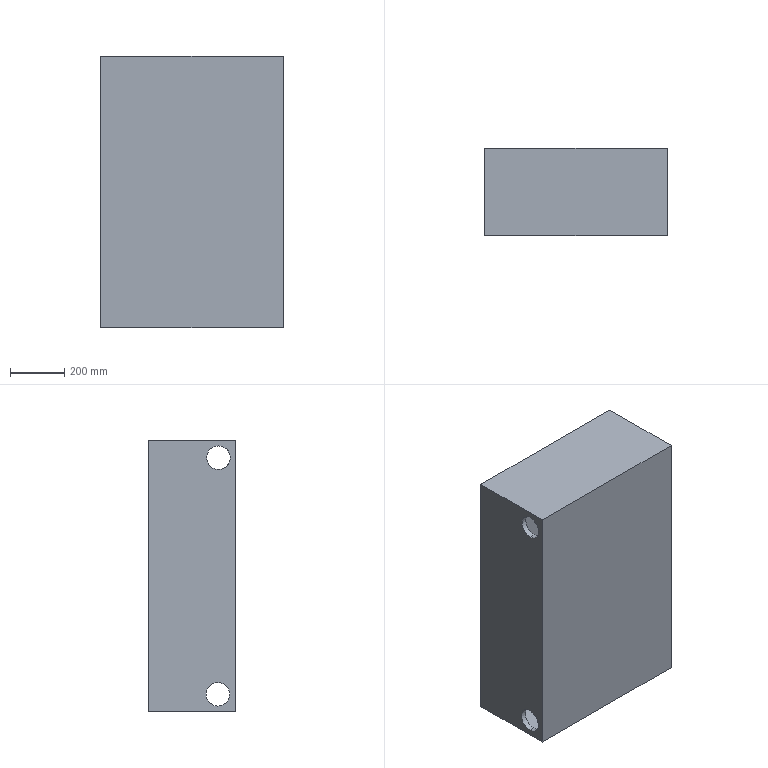Part | SolidWorks | features BaseBody 1 | 1 solid | 34 faces | box 670 x 320 x 1000 mm | volume 50005072 mm3 | cylinder 17 | plane 17 | commonest cylinder face diameters 60 x8 86.602 x7 110 x2
STEP:
#1=CARTESIAN_POINT('',(3055.278,1085.583,108.301));
#2=VERTEX_POINT('',#1);
#3=CARTESIAN_POINT('',(3055.278,1085.583,21.699));
#4=VERTEX_POINT('',#3);
#5=CARTESIAN_POINT('',(3055.278,1085.583,65.));
#6=DIRECTION('',(1.,0.,0.));
#7=DIRECTION('',(0.,0.,-1.));
#8=AXIS2_PLACEMENT_3D('',#5,#6,#7);
#9=CIRCLE('',#8,43.301);
#10=EDGE_CURVE('',#2,#4,#9,.T.);
#11=ORIENTED_EDGE('',*,*,#10,.T.);
#12=CARTESIAN_POINT('',(3035.278,1085.583,21.699));
#13=VERTEX_POINT('',#12);
#14=CARTESIAN_POINT('',(3705.278,1085.583,21.699));
#15=DIRECTION('',(-1.,0.,0.));
#16=VECTOR('',#15,1000.);
#17=LINE('',#14,#16);
#18=EDGE_CURVE('',#4,#13,#17,.T.);
#19=ORIENTED_EDGE('',*,*,#18,.T.);
#20=CARTESIAN_POINT('',(3035.278,1085.583,108.301));
#21=VERTEX_POINT('',#20);
#22=CARTESIAN_POINT('',(3035.278,1085.583,65.));
#23=DIRECTION('',(-1.,0.,0.));
#24=DIRECTION('',(0.,0.,1.));
#25=AXIS2_PLACEMENT_3D('',#22,#23,#24);
#26=CIRCLE('',#25,43.301);
#27=EDGE_CURVE('',#13,#21,#26,.T.);
#28=ORIENTED_EDGE('',*,*,#27,.T.);
#29=CARTESIAN_POINT('',(3705.278,1085.583,108.301));
#30=DIRECTION('',(-1.,0.,0.));
#31=VECTOR('',#30,1000.);
#32=LINE('',#29,#31);
#33=EDGE_CURVE('',#2,#21,#32,.T.);
#34=ORIENTED_EDGE('',*,*,#33,.F.);
#35=EDGE_LOOP('',(#11,#19,#28,#34));
#36=FACE_OUTER_BOUND('',#35,.T.);
#37=CARTESIAN_POINT('',(3705.278,1085.583,65.));
#38=DIRECTION('',(-1.,0.,0.));
#39=DIRECTION('',(0.,0.,1.));
#40=AXIS2_PLACEMENT_3D('',#37,#38,#39);
#41=CYLINDRICAL_SURFACE('',#40,43.301);
#42=ADVANCED_FACE('',(#36),#41,.F.);
#43=CARTESIAN_POINT('',(3705.278,1085.583,21.699));
#44=VERTEX_POINT('',#43);
#45=CARTESIAN_POINT('',(3705.278,1085.583,108.301));
#46=VERTEX_POINT('',#45);
#47=CARTESIAN_POINT('',(3705.278,1085.583,65.));
#48=DIRECTION('',(-1.,0.,0.));
#49=DIRECTION('',(0.,0.,1.));
#50=AXIS2_PLACEMENT_3D('',#47,#48,#49);
#51=CIRCLE('',#50,43.301);
#52=EDGE_CURVE('',#44,#46,#51,.T.);
#53=ORIENTED_EDGE('',*,*,#52,.F.);
#54=CARTESIAN_POINT('',(3685.278,1085.583,21.699));
#55=VERTEX_POINT('',#54);
#56=CARTESIAN_POINT('',(3705.278,1085.583,21.699));
#57=DIRECTION('',(-1.,0.,0.));
#58=VECTOR('',#57,1000.);
#59=LINE('',#56,#58);
#60=EDGE_CURVE('',#44,#55,#59,.T.);
#61=ORIENTED_EDGE('',*,*,#60,.T.);
#62=CARTESIAN_POINT('',(3685.278,1085.583,108.301));
#63=VERTEX_POINT('',#62);
#64=CARTESIAN_POINT('',(3685.278,1085.583,65.));
#65=DIRECTION('',(-1.,0.,0.));
#66=DIRECTION('',(0.,0.,1.));
#67=AXIS2_PLACEMENT_3D('',#64,#65,#66);
#68=CIRCLE('',#67,43.301);
#69=EDGE_CURVE('',#55,#63,#68,.T.);
#70=ORIENTED_EDGE('',*,*,#69,.T.);
#71=CARTESIAN_POINT('',(3705.278,1085.583,108.301));
#72=DIRECTION('',(-1.,0.,0.));
#73=VECTOR('',#72,1000.);
#74=LINE('',#71,#73);
#75=EDGE_CURVE('',#46,#63,#74,.T.);
#76=ORIENTED_EDGE('',*,*,#75,.F.);
#77=EDGE_LOOP('',(#53,#61,#70,#76));
#78=FACE_OUTER_BOUND('',#77,.T.);
#79=CARTESIAN_POINT('',(3705.278,1085.583,65.));
#80=DIRECTION('',(-1.,0.,0.));
#81=DIRECTION('',(0.,0.,1.));
#82=AXIS2_PLACEMENT_3D('',#79,#80,#81);
#83=CYLINDRICAL_SURFACE('',#82,43.301);
#84=ADVANCED_FACE('',(#78),#83,.F.);
#85=CARTESIAN_POINT('',(3705.278,1083.32,891.699));
#86=VERTEX_POINT('',#85);
#87=CARTESIAN_POINT('',(3705.278,1083.32,978.301));
#88=VERTEX_POINT('',#87);
#89=CARTESIAN_POINT('',(3705.278,1083.32,935.));
#90=DIRECTION('',(-1.,0.,0.));
#91=DIRECTION('',(0.,0.,1.));
#92=AXIS2_PLACEMENT_3D('',#89,#90,#91);
#93=CIRCLE('',#92,43.301);
#94=EDGE_CURVE('',#86,#88,#93,.T.);
#95=ORIENTED_EDGE('',*,*,#94,.F.);
#96=CARTESIAN_POINT('',(3685.278,1083.32,891.699));
#97=VERTEX_POINT('',#96);
#98=CARTESIAN_POINT('',(3705.278,1083.32,891.699));
#99=DIRECTION('',(-1.,0.,0.));
#100=VECTOR('',#99,1000.);
#101=LINE('',#98,#100);
#102=EDGE_CURVE('',#86,#97,#101,.T.);
#103=ORIENTED_EDGE('',*,*,#102,.T.);
#104=CARTESIAN_POINT('',(3685.278,1040.583,928.037));
#105=VERTEX_POINT('',#104);
#106=CARTESIAN_POINT('',(3685.278,1083.32,935.));
#107=DIRECTION('',(-1.,0.,0.));
#108=DIRECTION('',(0.,0.,1.));
#109=AXIS2_PLACEMENT_3D('',#106,#107,#108);
#110=CIRCLE('',#109,43.301);
#111=EDGE_CURVE('',#97,#105,#110,.T.);
#112=ORIENTED_EDGE('',*,*,#111,.T.);
#113=CARTESIAN_POINT('',(3055.278,1040.583,928.037));
#114=VERTEX_POINT('',#113);
#115=CARTESIAN_POINT('',(3705.278,1040.583,928.037));
#116=DIRECTION('',(-1.,0.,0.));
#117=VECTOR('',#116,1000.);
#118=LINE('',#115,#117);
#119=EDGE_CURVE('',#105,#114,#118,.T.);
#120=ORIENTED_EDGE('',*,*,#119,.T.);
#121=CARTESIAN_POINT('',(3055.278,1083.32,891.699));
#122=VERTEX_POINT('',#121);
#123=CARTESIAN_POINT('',(3055.278,1083.32,935.));
#124=DIRECTION('',(1.,0.,0.));
#125=DIRECTION('',(0.,0.,-1.));
#126=AXIS2_PLACEMENT_3D('',#123,#124,#125);
#127=CIRCLE('',#126,43.301);
#128=EDGE_CURVE('',#114,#122,#127,.T.);
#129=ORIENTED_EDGE('',*,*,#128,.T.);
#130=CARTESIAN_POINT('',(3035.278,1083.32,891.699));
#131=VERTEX_POINT('',#130);
#132=CARTESIAN_POINT('',(3705.278,1083.32,891.699));
#133=DIRECTION('',(-1.,0.,0.));
#134=VECTOR('',#133,1000.);
#135=LINE('',#132,#134);
#136=EDGE_CURVE('',#122,#131,#135,.T.);
#137=ORIENTED_EDGE('',*,*,#136,.T.);
#138=CARTESIAN_POINT('',(3035.278,1083.32,978.301));
#139=VERTEX_POINT('',#138);
#140=CARTESIAN_POINT('',(3035.278,1083.32,935.));
#141=DIRECTION('',(-1.,0.,0.));
#142=DIRECTION('',(0.,0.,1.));
#143=AXIS2_PLACEMENT_3D('',#140,#141,#142);
#144=CIRCLE('',#143,43.301);
#145=EDGE_CURVE('',#131,#139,#144,.T.);
#146=ORIENTED_EDGE('',*,*,#145,.T.);
#147=CARTESIAN_POINT('',(3055.278,1083.32,978.301));
#148=VERTEX_POINT('',#147);
#149=CARTESIAN_POINT('',(3705.278,1083.32,978.301));
#150=DIRECTION('',(-1.,0.,0.));
#151=VECTOR('',#150,1000.);
#152=LINE('',#149,#151);
#153=EDGE_CURVE('',#148,#139,#152,.T.);
#154=ORIENTED_EDGE('',*,*,#153,.F.);
#155=CARTESIAN_POINT('',(3055.278,1040.583,941.963));
#156=VERTEX_POINT('',#155);
#157=CARTESIAN_POINT('',(3055.278,1083.32,935.));
#158=DIRECTION('',(1.,0.,0.));
#159=DIRECTION('',(0.,0.,-1.));
#160=AXIS2_PLACEMENT_3D('',#157,#158,#159);
#161=CIRCLE('',#160,43.301);
#162=EDGE_CURVE('',#148,#156,#161,.T.);
#163=ORIENTED_EDGE('',*,*,#162,.T.);
#164=CARTESIAN_POINT('',(3685.278,1040.583,941.963));
#165=VERTEX_POINT('',#164);
#166=CARTESIAN_POINT('',(3705.278,1040.583,941.963));
#167=DIRECTION('',(1.,0.,0.));
#168=VECTOR('',#167,1000.);
#169=LINE('',#166,#168);
#170=EDGE_CURVE('',#156,#165,#169,.T.);
#171=ORIENTED_EDGE('',*,*,#170,.T.);
#172=CARTESIAN_POINT('',(3685.278,1083.32,978.301));
#173=VERTEX_POINT('',#172);
#174=CARTESIAN_POINT('',(3685.278,1083.32,935.));
#175=DIRECTION('',(-1.,0.,0.));
#176=DIRECTION('',(0.,0.,1.));
#177=AXIS2_PLACEMENT_3D('',#174,#175,#176);
#178=CIRCLE('',#177,43.301);
#179=EDGE_CURVE('',#165,#173,#178,.T.);
#180=ORIENTED_EDGE('',*,*,#179,.T.);
#181=CARTESIAN_POINT('',(3705.278,1083.32,978.301));
#182=DIRECTION('',(-1.,0.,0.));
#183=VECTOR('',#182,1000.);
#184=LINE('',#181,#183);
#185=EDGE_CURVE('',#88,#173,#184,.T.);
#186=ORIENTED_EDGE('',*,*,#185,.F.);
#187=EDGE_LOOP('',(#95,#103,#112,#120,#129,#137,#146,#154,#163,#171,#180,#186));
#188=FACE_OUTER_BOUND('',#187,.T.);
#189=CARTESIAN_POINT('',(3705.278,1083.32,935.));
#190=DIRECTION('',(-1.,0.,0.));
#191=DIRECTION('',(0.,0.,1.));
#192=AXIS2_PLACEMENT_3D('',#189,#190,#191);
#193=CYLINDRICAL_SURFACE('',#192,43.301);
#194=ADVANCED_FACE('',(#188),#193,.F.);
#195=ORIENTED_EDGE('',*,*,#102,.F.);
#196=CARTESIAN_POINT('',(3705.278,1083.32,935.));
#197=DIRECTION('',(-1.,0.,0.));
#198=DIRECTION('',(0.,0.,1.));
#199=AXIS2_PLACEMENT_3D('',#196,#197,#198);
#200=CIRCLE('',#199,43.301);
#201=EDGE_CURVE('',#88,#86,#200,.T.);
#202=ORIENTED_EDGE('',*,*,#201,.F.);
#203=ORIENTED_EDGE('',*,*,#185,.T.);
#204=CARTESIAN_POINT('',(3685.278,1083.32,935.));
#205=DIRECTION('',(-1.,0.,0.));
#206=DIRECTION('',(0.,0.,1.));
#207=AXIS2_PLACEMENT_3D('',#204,#205,#206);
#208=CIRCLE('',#207,43.301);
#209=EDGE_CURVE('',#173,#97,#208,.T.);
#210=ORIENTED_EDGE('',*,*,#209,.T.);
#211=EDGE_LOOP('',(#195,#202,#203,#210));
#212=FACE_OUTER_BOUND('',#211,.T.);
#213=CARTESIAN_POINT('',(3705.278,1083.32,935.));
#214=DIRECTION('',(-1.,0.,0.));
#215=DIRECTION('',(0.,0.,1.));
#216=AXIS2_PLACEMENT_3D('',#213,#214,#215);
#217=CYLINDRICAL_SURFACE('',#216,43.301);
#218=ADVANCED_FACE('',(#212),#217,.F.);
#219=CARTESIAN_POINT('',(3115.278,1310.583,950.));
#220=VERTEX_POINT('',#219);
#221=CARTESIAN_POINT('',(3055.278,1310.583,950.));
#222=VERTEX_POINT('',#221);
#223=CARTESIAN_POINT('',(3085.278,1310.583,950.));
#224=DIRECTION('',(0.,1.,0.));
#225=DIRECTION('',(-1.,0.,0.));
#226=AXIS2_PLACEMENT_3D('',#223,#224,#225);
#227=CIRCLE('',#226,30.);
#228=EDGE_CURVE('',#220,#222,#227,.T.);
#229=ORIENTED_EDGE('',*,*,#228,.F.);
#230=CARTESIAN_POINT('',(3115.278,1340.583,950.));
#231=VERTEX_POINT('',#230);
#232=CARTESIAN_POINT('',(3115.278,1310.583,950.));
#233=DIRECTION('',(0.,1.,0.));
#234=VECTOR('',#233,1000.);
#235=LINE('',#232,#234);
#236=EDGE_CURVE('',#220,#231,#235,.T.);
#237=ORIENTED_EDGE('',*,*,#236,.T.);
#238=CARTESIAN_POINT('',(3055.278,1340.583,950.));
#239=VERTEX_POINT('',#238);
#240=CARTESIAN_POINT('',(3085.278,1340.583,950.));
#241=DIRECTION('',(0.,1.,0.));
#242=DIRECTION('',(-1.,0.,0.));
#243=AXIS2_PLACEMENT_3D('',#240,#241,#242);
#244=CIRCLE('',#243,30.);
#245=EDGE_CURVE('',#231,#239,#244,.T.);
#246=ORIENTED_EDGE('',*,*,#245,.T.);
#247=CARTESIAN_POINT('',(3055.278,1310.583,950.));
#248=DIRECTION('',(0.,1.,0.));
#249=VECTOR('',#248,1000.);
#250=LINE('',#247,#249);
#251=EDGE_CURVE('',#222,#239,#250,.T.);
#252=ORIENTED_EDGE('',*,*,#251,.F.);
#253=EDGE_LOOP('',(#229,#237,#246,#252));
#254=FACE_OUTER_BOUND('',#253,.T.);
#255=CARTESIAN_POINT('',(3085.278,1310.583,950.));
#256=DIRECTION('',(0.,1.,0.));
#257=DIRECTION('',(-1.,0.,0.));
#258=AXIS2_PLACEMENT_3D('',#255,#256,#257);
#259=CYLINDRICAL_SURFACE('',#258,30.);
#260=ADVANCED_FACE('',(#254),#259,.F.);
#261=CARTESIAN_POINT('',(3685.278,1310.583,50.));
#262=VERTEX_POINT('',#261);
#263=CARTESIAN_POINT('',(3655.278,1310.583,20.));
#264=VERTEX_POINT('',#263);
#265=CARTESIAN_POINT('',(3655.278,1310.583,50.));
#266=DIRECTION('',(0.,1.,0.));
#267=DIRECTION('',(1.,0.,0.));
#268=AXIS2_PLACEMENT_3D('',#265,#266,#267);
#269=CIRCLE('',#268,30.);
#270=EDGE_CURVE('',#262,#264,#269,.T.);
#271=ORIENTED_EDGE('',*,*,#270,.F.);
#272=CARTESIAN_POINT('',(3685.278,1340.583,50.));
#273=VERTEX_POINT('',#272);
#274=CARTESIAN_POINT('',(3685.278,1310.583,50.));
#275=DIRECTION('',(0.,1.,0.));
#276=VECTOR('',#275,1000.);
#277=LINE('',#274,#276);
#278=EDGE_CURVE('',#262,#273,#277,.T.);
#279=ORIENTED_EDGE('',*,*,#278,.T.);
#280=CARTESIAN_POINT('',(3625.278,1340.583,50.));
#281=VERTEX_POINT('',#280);
#282=CARTESIAN_POINT('',(3655.278,1340.583,50.));
#283=DIRECTION('',(0.,1.,0.));
#284=DIRECTION('',(1.,0.,0.));
#285=AXIS2_PLACEMENT_3D('',#282,#283,#284);
#286=CIRCLE('',#285,30.);
#287=EDGE_CURVE('',#273,#281,#286,.T.);
#288=ORIENTED_EDGE('',*,*,#287,.T.);
#289=CARTESIAN_POINT('',(3625.278,1310.583,50.));
#290=VERTEX_POINT('',#289);
#291=CARTESIAN_POINT('',(3625.278,1310.583,50.));
#292=DIRECTION('',(0.,1.,0.));
#293=VECTOR('',#292,1000.);
#294=LINE('',#291,#293);
#295=EDGE_CURVE('',#290,#281,#294,.T.);
#296=ORIENTED_EDGE('',*,*,#295,.F.);
#297=CARTESIAN_POINT('',(3655.278,1310.583,50.));
#298=DIRECTION('',(0.,1.,0.));
#299=DIRECTION('',(1.,0.,0.));
#300=AXIS2_PLACEMENT_3D('',#297,#298,#299);
#301=CIRCLE('',#300,30.);
#302=EDGE_CURVE('',#264,#290,#301,.T.);
#303=ORIENTED_EDGE('',*,*,#302,.F.);
#304=EDGE_LOOP('',(#271,#279,#288,#296,#303));
#305=FACE_OUTER_BOUND('',#304,.T.);
#306=CARTESIAN_POINT('',(3655.278,1310.583,50.));
#307=DIRECTION('',(0.,1.,0.));
#308=DIRECTION('',(-1.,0.,0.));
#309=AXIS2_PLACEMENT_3D('',#306,#307,#308);
#310=CYLINDRICAL_SURFACE('',#309,30.);
#311=ADVANCED_FACE('',(#305),#310,.F.);
#312=CARTESIAN_POINT('',(3685.278,1310.583,950.));
#313=VERTEX_POINT('',#312);
#314=CARTESIAN_POINT('',(3625.278,1310.583,950.));
#315=VERTEX_POINT('',#314);
#316=CARTESIAN_POINT('',(3655.278,1310.583,950.));
#317=DIRECTION('',(0.,1.,0.));
#318=DIRECTION('',(-1.,0.,0.));
#319=AXIS2_PLACEMENT_3D('',#316,#317,#318);
#320=CIRCLE('',#319,30.);
#321=EDGE_CURVE('',#313,#315,#320,.T.);
#322=ORIENTED_EDGE('',*,*,#321,.F.);
#323=CARTESIAN_POINT('',(3685.278,1340.583,950.));
#324=VERTEX_POINT('',#323);
#325=CARTESIAN_POINT('',(3685.278,1310.583,950.));
#326=DIRECTION('',(0.,1.,0.));
#327=VECTOR('',#326,1000.);
#328=LINE('',#325,#327);
#329=EDGE_CURVE('',#313,#324,#328,.T.);
#330=ORIENTED_EDGE('',*,*,#329,.T.);
#331=CARTESIAN_POINT('',(3625.278,1340.583,950.));
#332=VERTEX_POINT('',#331);
#333=CARTESIAN_POINT('',(3655.278,1340.583,950.));
#334=DIRECTION('',(0.,1.,0.));
#335=DIRECTION('',(-1.,0.,0.));
#336=AXIS2_PLACEMENT_3D('',#333,#334,#335);
#337=CIRCLE('',#336,30.);
#338=EDGE_CURVE('',#324,#332,#337,.T.);
#339=ORIENTED_EDGE('',*,*,#338,.T.);
#340=CARTESIAN_POINT('',(3625.278,1310.583,950.));
#341=DIRECTION('',(0.,1.,0.));
#342=VECTOR('',#341,1000.);
#343=LINE('',#340,#342);
#344=EDGE_CURVE('',#315,#332,#343,.T.);
#345=ORIENTED_EDGE('',*,*,#344,.F.);
#346=EDGE_LOOP('',(#322,#330,#339,#345));
#347=FACE_OUTER_BOUND('',#346,.T.);
#348=CARTESIAN_POINT('',(3655.278,1310.583,950.));
#349=DIRECTION('',(0.,1.,0.));
#350=DIRECTION('',(-1.,0.,0.));
#351=AXIS2_PLACEMENT_3D('',#348,#349,#350);
#352=CYLINDRICAL_SURFACE('',#351,30.);
#353=ADVANCED_FACE('',(#347),#352,.F.);
#354=CARTESIAN_POINT('',(3115.278,1310.583,50.));
#355=VERTEX_POINT('',#354);
#356=CARTESIAN_POINT('',(3085.278,1310.583,20.));
#357=VERTEX_POINT('',#356);
#358=CARTESIAN_POINT('',(3085.278,1310.583,50.));
#359=DIRECTION('',(0.,1.,0.));
#360=DIRECTION('',(1.,0.,0.));
#361=AXIS2_PLACEMENT_3D('',#358,#359,#360);
#362=CIRCLE('',#361,30.);
#363=EDGE_CURVE('',#355,#357,#362,.T.);
#364=ORIENTED_EDGE('',*,*,#363,.F.);
#365=CARTESIAN_POINT('',(3115.278,1340.583,50.));
#366=VERTEX_POINT('',#365);
#367=CARTESIAN_POINT('',(3115.278,1310.583,50.));
#368=DIRECTION('',(0.,1.,0.));
#369=VECTOR('',#368,1000.);
#370=LINE('',#367,#369);
#371=EDGE_CURVE('',#355,#366,#370,.T.);
#372=ORIENTED_EDGE('',*,*,#371,.T.);
#373=CARTESIAN_POINT('',(3055.278,1340.583,50.));
#374=VERTEX_POINT('',#373);
#375=CARTESIAN_POINT('',(3085.278,1340.583,50.));
#376=DIRECTION('',(0.,1.,0.));
#377=DIRECTION('',(1.,0.,0.));
#378=AXIS2_PLACEMENT_3D('',#375,#376,#377);
#379=CIRCLE('',#378,30.);
#380=EDGE_CURVE('',#366,#374,#379,.T.);
#381=ORIENTED_EDGE('',*,*,#380,.T.);
#382=CARTESIAN_POINT('',(3055.278,1310.583,50.));
#383=VERTEX_POINT('',#382);
#384=CARTESIAN_POINT('',(3055.278,1310.583,50.));
#385=DIRECTION('',(0.,1.,0.));
#386=VECTOR('',#385,1000.);
#387=LINE('',#384,#386);
#388=EDGE_CURVE('',#383,#374,#387,.T.);
#389=ORIENTED_EDGE('',*,*,#388,.F.);
#390=CARTESIAN_POINT('',(3085.278,1310.583,50.));
#391=DIRECTION('',(0.,1.,0.));
#392=DIRECTION('',(1.,0.,0.));
#393=AXIS2_PLACEMENT_3D('',#390,#391,#392);
#394=CIRCLE('',#393,30.);
#395=EDGE_CURVE('',#357,#383,#394,.T.);
#396=ORIENTED_EDGE('',*,*,#395,.F.);
#397=EDGE_LOOP('',(#364,#372,#381,#389,#396));
#398=FACE_OUTER_BOUND('',#397,.T.);
#399=CARTESIAN_POINT('',(3085.278,1310.583,50.));
#400=DIRECTION('',(0.,1.,0.));
#401=DIRECTION('',(-1.,0.,0.));
#402=AXIS2_PLACEMENT_3D('',#399,#400,#401);
#403=CYLINDRICAL_SURFACE('',#402,30.);
#404=ADVANCED_FACE('',(#398),#403,.F.);
#405=CARTESIAN_POINT('',(3425.278,1310.583,500.));
#406=VERTEX_POINT('',#405);
#407=CARTESIAN_POINT('',(3315.278,1310.583,500.));
#408=VERTEX_POINT('',#407);
#409=CARTESIAN_POINT('',(3370.278,1310.583,500.));
#410=DIRECTION('',(0.,1.,0.));
#411=DIRECTION('',(-1.,0.,0.));
#412=AXIS2_PLACEMENT_3D('',#409,#410,#411);
#413=CIRCLE('',#412,55.);
#414=EDGE_CURVE('',#406,#408,#413,.T.);
#415=ORIENTED_EDGE('',*,*,#414,.F.);
#416=CARTESIAN_POINT('',(3425.278,1340.583,500.));
#417=VERTEX_POINT('',#416);
#418=CARTESIAN_POINT('',(3425.278,1310.583,500.));
#419=DIRECTION('',(0.,1.,0.));
#420=VECTOR('',#419,1000.);
#421=LINE('',#418,#420);
#422=EDGE_CURVE('',#406,#417,#421,.T.);
#423=ORIENTED_EDGE('',*,*,#422,.T.);
#424=CARTESIAN_POINT('',(3315.278,1340.583,500.));
#425=VERTEX_POINT('',#424);
#426=CARTESIAN_POINT('',(3370.278,1340.583,500.));
#427=DIRECTION('',(0.,1.,0.));
#428=DIRECTION('',(-1.,0.,0.));
#429=AXIS2_PLACEMENT_3D('',#426,#427,#428);
#430=CIRCLE('',#429,55.);
#431=EDGE_CURVE('',#417,#425,#430,.T.);
#432=ORIENTED_EDGE('',*,*,#431,.T.);
#433=CARTESIAN_POINT('',(3315.278,1310.583,500.));
#434=DIRECTION('',(0.,1.,0.));
#435=VECTOR('',#434,1000.);
#436=LINE('',#433,#435);
#437=EDGE_CURVE('',#408,#425,#436,.T.);
#438=ORIENTED_EDGE('',*,*,#437,.F.);
#439=EDGE_LOOP('',(#415,#423,#432,#438));
#440=FACE_OUTER_BOUND('',#439,.T.);
#441=CARTESIAN_POINT('',(3370.278,1310.583,500.));
#442=DIRECTION('',(0.,1.,0.));
#443=DIRECTION('',(-1.,0.,0.));
#444=AXIS2_PLACEMENT_3D('',#441,#442,#443);
#445=CYLINDRICAL_SURFACE('',#444,55.);
#446=ADVANCED_FACE('',(#440),#445,.F.);
#447=ORIENTED_EDGE('',*,*,#119,.F.);
#448=CARTESIAN_POINT('',(3685.278,1040.583,20.));
#449=VERTEX_POINT('',#448);
#450=CARTESIAN_POINT('',(3685.278,1040.583,1000.));
#451=DIRECTION('',(0.,0.,-1.));
#452=VECTOR('',#451,1000.);
#453=LINE('',#450,#452);
#454=EDGE_CURVE('',#105,#449,#453,.T.);
#455=ORIENTED_EDGE('',*,*,#454,.T.);
#456=CARTESIAN_POINT('',(3055.278,1040.583,20.));
#457=VERTEX_POINT('',#456);
#458=CARTESIAN_POINT('',(0.,1040.583,20.));
#459=DIRECTION('',(1.,0.,0.));
#460=VECTOR('',#459,1000.);
#461=LINE('',#458,#460);
#462=EDGE_CURVE('',#457,#449,#461,.T.);
#463=ORIENTED_EDGE('',*,*,#462,.F.);
#464=CARTESIAN_POINT('',(3055.278,1040.583,1000.));
#465=DIRECTION('',(0.,0.,-1.));
#466=VECTOR('',#465,1000.);
#467=LINE('',#464,#466);
#468=EDGE_CURVE('',#114,#457,#467,.T.);
#469=ORIENTED_EDGE('',*,*,#468,.F.);
#470=EDGE_LOOP('',(#447,#455,#463,#469));
#471=FACE_OUTER_BOUND('',#470,.T.);
#472=CARTESIAN_POINT('',(3035.278,1040.583,1000.));
#473=DIRECTION('',(0.,1.,0.));
#474=DIRECTION('',(0.,0.,1.));
#475=AXIS2_PLACEMENT_3D('',#472,#473,#474);
#476=PLANE('',#475);
#477=ADVANCED_FACE('',(#471),#476,.T.);
#478=CARTESIAN_POINT('',(3055.278,1310.583,980.));
#479=VERTEX_POINT('',#478);
#480=CARTESIAN_POINT('',(3055.278,1310.583,20.));
#481=DIRECTION('',(0.,0.,1.));
#482=VECTOR('',#481,1000.);
#483=LINE('',#480,#482);
#484=EDGE_CURVE('',#222,#479,#483,.T.);
#485=ORIENTED_EDGE('',*,*,#484,.F.);
#486=CARTESIAN_POINT('',(3085.278,1310.583,980.));
#487=VERTEX_POINT('',#486);
#488=CARTESIAN_POINT('',(3085.278,1310.583,950.));
#489=DIRECTION('',(0.,1.,0.));
#490=DIRECTION('',(-1.,0.,0.));
#491=AXIS2_PLACEMENT_3D('',#488,#489,#490);
#492=CIRCLE('',#491,30.);
#493=EDGE_CURVE('',#222,#487,#492,.T.);
#494=ORIENTED_EDGE('',*,*,#493,.T.);
#495=CARTESIAN_POINT('',(3055.278,1310.583,980.));
#496=DIRECTION('',(1.,0.,0.));
#497=VECTOR('',#496,1000.);
#498=LINE('',#495,#497);
#499=EDGE_CURVE('',#479,#487,#498,.T.);
#500=ORIENTED_EDGE('',*,*,#499,.F.);
#501=EDGE_LOOP('',(#485,#494,#500));
#502=FACE_OUTER_BOUND('',#501,.T.);
#503=CARTESIAN_POINT('',(0.,1310.583,0.));
#504=DIRECTION('',(0.,1.,0.));
#505=DIRECTION('',(-1.,0.,0.));
#506=AXIS2_PLACEMENT_3D('',#503,#504,#505);
#507=PLANE('',#506);
#508=ADVANCED_FACE('',(#502),#507,.F.);
#509=CARTESIAN_POINT('',(3685.278,1310.583,20.));
#510=VERTEX_POINT('',#509);
#511=CARTESIAN_POINT('',(3685.278,1310.583,980.));
#512=DIRECTION('',(0.,0.,-1.));
#513=VECTOR('',#512,1000.);
#514=LINE('',#511,#513);
#515=EDGE_CURVE('',#262,#510,#514,.T.);
#516=ORIENTED_EDGE('',*,*,#515,.F.);
#517=ORIENTED_EDGE('',*,*,#270,.T.);
#518=CARTESIAN_POINT('',(3685.278,1310.583,20.));
#519=DIRECTION('',(-1.,0.,0.));
#520=VECTOR('',#519,1000.);
#521=LINE('',#518,#520);
#522=EDGE_CURVE('',#510,#264,#521,.T.);
#523=ORIENTED_EDGE('',*,*,#522,.F.);
#524=EDGE_LOOP('',(#516,#517,#523));
#525=FACE_OUTER_BOUND('',#524,.T.);
#526=CARTESIAN_POINT('',(0.,1310.583,0.));
#527=DIRECTION('',(0.,1.,0.));
#528=DIRECTION('',(-1.,0.,0.));
#529=AXIS2_PLACEMENT_3D('',#526,#527,#528);
#530=PLANE('',#529);
#531=ADVANCED_FACE('',(#525),#530,.F.);
#532=CARTESIAN_POINT('',(3655.278,1310.583,980.));
#533=VERTEX_POINT('',#532);
#534=CARTESIAN_POINT('',(3685.278,1310.583,980.));
#535=VERTEX_POINT('',#534);
#536=CARTESIAN_POINT('',(3055.278,1310.583,980.));
#537=DIRECTION('',(1.,0.,0.));
#538=VECTOR('',#537,1000.);
#539=LINE('',#536,#538);
#540=EDGE_CURVE('',#533,#535,#539,.T.);
#541=ORIENTED_EDGE('',*,*,#540,.F.);
#542=CARTESIAN_POINT('',(3655.278,1310.583,950.));
#543=DIRECTION('',(0.,1.,0.));
#544=DIRECTION('',(-1.,0.,0.));
#545=AXIS2_PLACEMENT_3D('',#542,#543,#544);
#546=CIRCLE('',#545,30.);
#547=EDGE_CURVE('',#533,#313,#546,.T.);
#548=ORIENTED_EDGE('',*,*,#547,.T.);
#549=CARTESIAN_POINT('',(3685.278,1310.583,980.));
#550=DIRECTION('',(0.,0.,-1.));
#551=VECTOR('',#550,1000.);
#552=LINE('',#549,#551);
#553=EDGE_CURVE('',#535,#313,#552,.T.);
#554=ORIENTED_EDGE('',*,*,#553,.F.);
#555=EDGE_LOOP('',(#541,#548,#554));
#556=FACE_OUTER_BOUND('',#555,.T.);
#557=CARTESIAN_POINT('',(0.,1310.583,0.));
#558=DIRECTION('',(0.,1.,0.));
#559=DIRECTION('',(-1.,0.,0.));
#560=AXIS2_PLACEMENT_3D('',#557,#558,#559);
#561=PLANE('',#560);
#562=ADVANCED_FACE('',(#556),#561,.F.);
#563=CARTESIAN_POINT('',(3055.278,1310.583,20.));
#564=VERTEX_POINT('',#563);
#565=CARTESIAN_POINT('',(3685.278,1310.583,20.));
#566=DIRECTION('',(-1.,0.,0.));
#567=VECTOR('',#566,1000.);
#568=LINE('',#565,#567);
#569=EDGE_CURVE('',#357,#564,#568,.T.);
#570=ORIENTED_EDGE('',*,*,#569,.F.);
#571=ORIENTED_EDGE('',*,*,#395,.T.);
#572=CARTESIAN_POINT('',(3055.278,1310.583,20.));
#573=DIRECTION('',(0.,0.,1.));
#574=VECTOR('',#573,1000.);
#575=LINE('',#572,#574);
#576=EDGE_CURVE('',#564,#383,#575,.T.);
#577=ORIENTED_EDGE('',*,*,#576,.F.);
#578=EDGE_LOOP('',(#570,#571,#577));
#579=FACE_OUTER_BOUND('',#578,.T.);
#580=CARTESIAN_POINT('',(0.,1310.583,0.));
#581=DIRECTION('',(0.,1.,0.));
#582=DIRECTION('',(-1.,0.,0.));
#583=AXIS2_PLACEMENT_3D('',#580,#581,#582);
#584=PLANE('',#583);
#585=ADVANCED_FACE('',(#579),#584,.F.);
#586=CARTESIAN_POINT('',(3370.278,1310.583,500.));
#587=DIRECTION('',(0.,1.,0.));
#588=DIRECTION('',(-1.,0.,0.));
#589=AXIS2_PLACEMENT_3D('',#586,#587,#588);
#590=CIRCLE('',#589,55.);
#591=EDGE_CURVE('',#408,#406,#590,.T.);
#592=ORIENTED_EDGE('',*,*,#591,.T.);
#593=ORIENTED_EDGE('',*,*,#414,.T.);
#594=EDGE_LOOP('',(#592,#593));
#595=FACE_BOUND('',#594,.T.);
#596=CARTESIAN_POINT('',(3055.278,1310.583,980.));
#597=DIRECTION('',(1.,0.,0.));
#598=VECTOR('',#597,1000.);
#599=LINE('',#596,#598);
#600=EDGE_CURVE('',#487,#533,#599,.T.);
#601=ORIENTED_EDGE('',*,*,#600,.F.);
#602=CARTESIAN_POINT('',(3085.278,1310.583,950.));
#603=DIRECTION('',(0.,1.,0.));
#604=DIRECTION('',(-1.,0.,0.));
#605=AXIS2_PLACEMENT_3D('',#602,#603,#604);
#606=CIRCLE('',#605,30.);
#607=EDGE_CURVE('',#487,#220,#606,.T.);
#608=ORIENTED_EDGE('',*,*,#607,.T.);
#609=ORIENTED_EDGE('',*,*,#228,.T.);
#610=CARTESIAN_POINT('',(3055.278,1310.583,20.));
#611=DIRECTION('',(0.,0.,1.));
#612=VECTOR('',#611,1000.);
#613=LINE('',#610,#612);
#614=EDGE_CURVE('',#383,#222,#613,.T.);
#615=ORIENTED_EDGE('',*,*,#614,.F.);
#616=CARTESIAN_POINT('',(3085.278,1310.583,50.));
#617=DIRECTION('',(0.,1.,0.));
#618=DIRECTION('',(1.,0.,0.));
#619=AXIS2_PLACEMENT_3D('',#616,#617,#618);
#620=CIRCLE('',#619,30.);
#621=EDGE_CURVE('',#383,#355,#620,.T.);
#622=ORIENTED_EDGE('',*,*,#621,.T.);
#623=ORIENTED_EDGE('',*,*,#363,.T.);
#624=CARTESIAN_POINT('',(3685.278,1310.583,20.));
#625=DIRECTION('',(-1.,0.,0.));
#626=VECTOR('',#625,1000.);
#627=LINE('',#624,#626);
#628=EDGE_CURVE('',#264,#357,#627,.T.);
#629=ORIENTED_EDGE('',*,*,#628,.F.);
#630=ORIENTED_EDGE('',*,*,#302,.T.);
#631=CARTESIAN_POINT('',(3655.278,1310.583,50.));
#632=DIRECTION('',(0.,1.,0.));
#633=DIRECTION('',(1.,0.,0.));
#634=AXIS2_PLACEMENT_3D('',#631,#632,#633);
#635=CIRCLE('',#634,30.);
#636=EDGE_CURVE('',#290,#262,#635,.T.);
#637=ORIENTED_EDGE('',*,*,#636,.T.);
#638=CARTESIAN_POINT('',(3685.278,1310.583,980.));
#639=DIRECTION('',(0.,0.,-1.));
#640=VECTOR('',#639,1000.);
#641=LINE('',#638,#640);
#642=EDGE_CURVE('',#313,#262,#641,.T.);
#643=ORIENTED_EDGE('',*,*,#642,.F.);
#644=ORIENTED_EDGE('',*,*,#321,.T.);
#645=CARTESIAN_POINT('',(3655.278,1310.583,950.));
#646=DIRECTION('',(0.,1.,0.));
#647=DIRECTION('',(-1.,0.,0.));
#648=AXIS2_PLACEMENT_3D('',#645,#646,#647);
#649=CIRCLE('',#648,30.);
#650=EDGE_CURVE('',#315,#533,#649,.T.);
#651=ORIENTED_EDGE('',*,*,#650,.T.);
#652=EDGE_LOOP('',(#601,#608,#609,#615,#622,#623,#629,#630,#637,#643,#644,#651));
#653=FACE_OUTER_BOUND('',#652,.T.);
#654=CARTESIAN_POINT('',(0.,1310.583,0.));
#655=DIRECTION('',(0.,1.,0.));
#656=DIRECTION('',(-1.,0.,0.));
#657=AXIS2_PLACEMENT_3D('',#654,#655,#656);
#658=PLANE('',#657);
#659=ADVANCED_FACE('',(#595,#653),#658,.F.);
#660=ORIENTED_EDGE('',*,*,#170,.F.);
#661=CARTESIAN_POINT('',(3055.278,1040.583,980.));
#662=VERTEX_POINT('',#661);
#663=CARTESIAN_POINT('',(3055.278,1040.583,1000.));
#664=DIRECTION('',(0.,0.,-1.));
#665=VECTOR('',#664,1000.);
#666=LINE('',#663,#665);
#667=EDGE_CURVE('',#662,#156,#666,.T.);
#668=ORIENTED_EDGE('',*,*,#667,.F.);
#669=CARTESIAN_POINT('',(3685.278,1040.583,980.));
#670=VERTEX_POINT('',#669);
#671=CARTESIAN_POINT('',(0.,1040.583,980.));
#672=DIRECTION('',(1.,0.,0.));
#673=VECTOR('',#672,1000.);
#674=LINE('',#671,#673);
#675=EDGE_CURVE('',#662,#670,#674,.T.);
#676=ORIENTED_EDGE('',*,*,#675,.T.);
#677=CARTESIAN_POINT('',(3685.278,1040.583,1000.));
#678=DIRECTION('',(0.,0.,-1.));
#679=VECTOR('',#678,1000.);
#680=LINE('',#677,#679);
#681=EDGE_CURVE('',#670,#165,#680,.T.);
#682=ORIENTED_EDGE('',*,*,#681,.T.);
#683=EDGE_LOOP('',(#660,#668,#676,#682));
#684=FACE_OUTER_BOUND('',#683,.T.);
#685=CARTESIAN_POINT('',(3035.278,1040.583,1000.));
#686=DIRECTION('',(0.,1.,0.));
#687=DIRECTION('',(0.,0.,1.));
#688=AXIS2_PLACEMENT_3D('',#685,#686,#687);
#689=PLANE('',#688);
#690=ADVANCED_FACE('',(#684),#689,.T.);
#691=ORIENTED_EDGE('',*,*,#522,.T.);
#692=ORIENTED_EDGE('',*,*,#628,.T.);
#693=ORIENTED_EDGE('',*,*,#569,.T.);
#694=CARTESIAN_POINT('',(3055.278,0.,20.));
#695=DIRECTION('',(0.,-1.,0.));
#696=VECTOR('',#695,1000.);
#697=LINE('',#694,#696);
#698=EDGE_CURVE('',#564,#457,#697,.T.);
#699=ORIENTED_EDGE('',*,*,#698,.T.);
#700=ORIENTED_EDGE('',*,*,#462,.T.);
#701=CARTESIAN_POINT('',(3685.278,0.,20.));
#702=DIRECTION('',(0.,1.,0.));
#703=VECTOR('',#702,1000.);
#704=LINE('',#701,#703);
#705=EDGE_CURVE('',#449,#510,#704,.T.);
#706=ORIENTED_EDGE('',*,*,#705,.T.);
#707=EDGE_LOOP('',(#691,#692,#693,#699,#700,#706));
#708=FACE_OUTER_BOUND('',#707,.T.);
#709=CARTESIAN_POINT('',(0.,0.,20.));
#710=DIRECTION('',(0.,0.,-1.));
#711=DIRECTION('',(-1.,0.,0.));
#712=AXIS2_PLACEMENT_3D('',#709,#710,#711);
#713=PLANE('',#712);
#714=ADVANCED_FACE('',(#708),#713,.F.);
#715=CARTESIAN_POINT('',(3055.278,0.,980.));
#716=DIRECTION('',(0.,-1.,0.));
#717=VECTOR('',#716,1000.);
#718=LINE('',#715,#717);
#719=EDGE_CURVE('',#479,#662,#718,.T.);
#720=ORIENTED_EDGE('',*,*,#719,.F.);
#721=ORIENTED_EDGE('',*,*,#499,.T.);
#722=ORIENTED_EDGE('',*,*,#600,.T.);
#723=ORIENTED_EDGE('',*,*,#540,.T.);
#724=CARTESIAN_POINT('',(3685.278,0.,980.));
#725=DIRECTION('',(0.,1.,0.));
#726=VECTOR('',#725,1000.);
#727=LINE('',#724,#726);
#728=EDGE_CURVE('',#670,#535,#727,.T.);
#729=ORIENTED_EDGE('',*,*,#728,.F.);
#730=ORIENTED_EDGE('',*,*,#675,.F.);
#731=EDGE_LOOP('',(#720,#721,#722,#723,#729,#730));
#732=FACE_OUTER_BOUND('',#731,.T.);
#733=CARTESIAN_POINT('',(0.,0.,980.));
#734=DIRECTION('',(0.,0.,-1.));
#735=DIRECTION('',(-1.,0.,0.));
#736=AXIS2_PLACEMENT_3D('',#733,#734,#735);
#737=PLANE('',#736);
#738=ADVANCED_FACE('',(#732),#737,.T.);
#739=CARTESIAN_POINT('',(3685.278,1085.583,65.));
#740=DIRECTION('',(-1.,0.,0.));
#741=DIRECTION('',(0.,0.,1.));
#742=AXIS2_PLACEMENT_3D('',#739,#740,#741);
#743=CIRCLE('',#742,43.301);
#744=EDGE_CURVE('',#63,#55,#743,.T.);
#745=ORIENTED_EDGE('',*,*,#744,.F.);
#746=ORIENTED_EDGE('',*,*,#69,.F.);
#747=EDGE_LOOP('',(#745,#746));
#748=FACE_BOUND('',#747,.T.);
#749=ORIENTED_EDGE('',*,*,#179,.F.);
#750=ORIENTED_EDGE('',*,*,#681,.F.);
#751=ORIENTED_EDGE('',*,*,#728,.T.);
#752=ORIENTED_EDGE('',*,*,#553,.T.);
#753=ORIENTED_EDGE('',*,*,#642,.T.);
#754=ORIENTED_EDGE('',*,*,#515,.T.);
#755=ORIENTED_EDGE('',*,*,#705,.F.);
#756=ORIENTED_EDGE('',*,*,#454,.F.);
#757=ORIENTED_EDGE('',*,*,#111,.F.);
#758=ORIENTED_EDGE('',*,*,#209,.F.);
#759=EDGE_LOOP('',(#749,#750,#751,#752,#753,#754,#755,#756,#757,#758));
#760=FACE_OUTER_BOUND('',#759,.T.);
#761=CARTESIAN_POINT('',(3685.278,1320.583,1000.));
#762=DIRECTION('',(-1.,0.,0.));
#763=DIRECTION('',(0.,0.,1.));
#764=AXIS2_PLACEMENT_3D('',#761,#762,#763);
#765=PLANE('',#764);
#766=ADVANCED_FACE('',(#748,#760),#765,.T.);
#767=ORIENTED_EDGE('',*,*,#10,.F.);
#768=CARTESIAN_POINT('',(3055.278,1085.583,65.));
#769=DIRECTION('',(1.,0.,0.));
#770=DIRECTION('',(0.,0.,-1.));
#771=AXIS2_PLACEMENT_3D('',#768,#769,#770);
#772=CIRCLE('',#771,43.301);
#773=EDGE_CURVE('',#4,#2,#772,.T.);
#774=ORIENTED_EDGE('',*,*,#773,.F.);
#775=EDGE_LOOP('',(#767,#774));
#776=FACE_BOUND('',#775,.T.);
#777=ORIENTED_EDGE('',*,*,#128,.F.);
#778=ORIENTED_EDGE('',*,*,#468,.T.);
#779=ORIENTED_EDGE('',*,*,#698,.F.);
#780=ORIENTED_EDGE('',*,*,#576,.T.);
#781=ORIENTED_EDGE('',*,*,#614,.T.);
#782=ORIENTED_EDGE('',*,*,#484,.T.);
#783=ORIENTED_EDGE('',*,*,#719,.T.);
#784=ORIENTED_EDGE('',*,*,#667,.T.);
#785=ORIENTED_EDGE('',*,*,#162,.F.);
#786=CARTESIAN_POINT('',(3055.278,1083.32,935.));
#787=DIRECTION('',(1.,0.,0.));
#788=DIRECTION('',(0.,0.,-1.));
#789=AXIS2_PLACEMENT_3D('',#786,#787,#788);
#790=CIRCLE('',#789,43.301);
#791=EDGE_CURVE('',#122,#148,#790,.T.);
#792=ORIENTED_EDGE('',*,*,#791,.F.);
#793=EDGE_LOOP('',(#777,#778,#779,#780,#781,#782,#783,#784,#785,#792));
#794=FACE_OUTER_BOUND('',#793,.T.);
#795=CARTESIAN_POINT('',(3055.278,1320.583,1000.));
#796=DIRECTION('',(1.,0.,0.));
#797=DIRECTION('',(0.,0.,-1.));
#798=AXIS2_PLACEMENT_3D('',#795,#796,#797);
#799=PLANE('',#798);
#800=ADVANCED_FACE('',(#776,#794),#799,.T.);
#801=ORIENTED_EDGE('',*,*,#422,.F.);
#802=ORIENTED_EDGE('',*,*,#591,.F.);
#803=ORIENTED_EDGE('',*,*,#437,.T.);
#804=CARTESIAN_POINT('',(3370.278,1340.583,500.));
#805=DIRECTION('',(0.,1.,0.));
#806=DIRECTION('',(-1.,0.,0.));
#807=AXIS2_PLACEMENT_3D('',#804,#805,#806);
#808=CIRCLE('',#807,55.);
#809=EDGE_CURVE('',#425,#417,#808,.T.);
#810=ORIENTED_EDGE('',*,*,#809,.T.);
#811=EDGE_LOOP('',(#801,#802,#803,#810));
#812=FACE_OUTER_BOUND('',#811,.T.);
#813=CARTESIAN_POINT('',(3370.278,1310.583,500.));
#814=DIRECTION('',(0.,1.,0.));
#815=DIRECTION('',(-1.,0.,0.));
#816=AXIS2_PLACEMENT_3D('',#813,#814,#815);
#817=CYLINDRICAL_SURFACE('',#816,55.);
#818=ADVANCED_FACE('',(#812),#817,.F.);
#819=CARTESIAN_POINT('',(3085.278,1340.583,950.));
#820=DIRECTION('',(0.,1.,0.));
#821=DIRECTION('',(-1.,0.,0.));
#822=AXIS2_PLACEMENT_3D('',#819,#820,#821);
#823=CIRCLE('',#822,30.);
#824=EDGE_CURVE('',#239,#231,#823,.T.);
#825=ORIENTED_EDGE('',*,*,#824,.F.);
#826=ORIENTED_EDGE('',*,*,#245,.F.);
#827=EDGE_LOOP('',(#825,#826));
#828=FACE_BOUND('',#827,.T.);
#829=CARTESIAN_POINT('',(3655.278,1340.583,50.));
#830=DIRECTION('',(0.,1.,0.));
#831=DIRECTION('',(1.,0.,0.));
#832=AXIS2_PLACEMENT_3D('',#829,#830,#831);
#833=CIRCLE('',#832,30.);
#834=EDGE_CURVE('',#281,#273,#833,.T.);
#835=ORIENTED_EDGE('',*,*,#834,.F.);
#836=ORIENTED_EDGE('',*,*,#287,.F.);
#837=EDGE_LOOP('',(#835,#836));
#838=FACE_BOUND('',#837,.T.);
#839=CARTESIAN_POINT('',(3655.278,1340.583,950.));
#840=DIRECTION('',(0.,1.,0.));
#841=DIRECTION('',(-1.,0.,0.));
#842=AXIS2_PLACEMENT_3D('',#839,#840,#841);
#843=CIRCLE('',#842,30.);
#844=EDGE_CURVE('',#332,#324,#843,.T.);
#845=ORIENTED_EDGE('',*,*,#844,.F.);
#846=ORIENTED_EDGE('',*,*,#338,.F.);
#847=EDGE_LOOP('',(#845,#846));
#848=FACE_BOUND('',#847,.T.);
#849=CARTESIAN_POINT('',(3085.278,1340.583,50.));
#850=DIRECTION('',(0.,1.,0.));
#851=DIRECTION('',(1.,0.,0.));
#852=AXIS2_PLACEMENT_3D('',#849,#850,#851);
#853=CIRCLE('',#852,30.);
#854=EDGE_CURVE('',#374,#366,#853,.T.);
#855=ORIENTED_EDGE('',*,*,#854,.F.);
#856=ORIENTED_EDGE('',*,*,#380,.F.);
#857=EDGE_LOOP('',(#855,#856));
#858=FACE_BOUND('',#857,.T.);
#859=ORIENTED_EDGE('',*,*,#809,.F.);
#860=ORIENTED_EDGE('',*,*,#431,.F.);
#861=EDGE_LOOP('',(#859,#860));
#862=FACE_BOUND('',#861,.T.);
#863=CARTESIAN_POINT('',(3705.278,1340.583,0.));
#864=VERTEX_POINT('',#863);
#865=CARTESIAN_POINT('',(3035.278,1340.583,0.));
#866=VERTEX_POINT('',#865);
#867=CARTESIAN_POINT('',(3035.278,1340.583,0.));
#868=DIRECTION('',(-1.,0.,0.));
#869=VECTOR('',#868,1000.);
#870=LINE('',#867,#869);
#871=EDGE_CURVE('',#864,#866,#870,.T.);
#872=ORIENTED_EDGE('',*,*,#871,.T.);
#873=CARTESIAN_POINT('',(3035.278,1340.583,1000.));
#874=VERTEX_POINT('',#873);
#875=CARTESIAN_POINT('',(3035.278,1340.583,1000.));
#876=DIRECTION('',(0.,0.,-1.));
#877=VECTOR('',#876,1000.);
#878=LINE('',#875,#877);
#879=EDGE_CURVE('',#874,#866,#878,.T.);
#880=ORIENTED_EDGE('',*,*,#879,.F.);
#881=CARTESIAN_POINT('',(3705.278,1340.583,1000.));
#882=VERTEX_POINT('',#881);
#883=CARTESIAN_POINT('',(3035.278,1340.583,1000.));
#884=DIRECTION('',(-1.,0.,0.));
#885=VECTOR('',#884,1000.);
#886=LINE('',#883,#885);
#887=EDGE_CURVE('',#882,#874,#886,.T.);
#888=ORIENTED_EDGE('',*,*,#887,.F.);
#889=CARTESIAN_POINT('',(3705.278,1340.583,1000.));
#890=DIRECTION('',(0.,0.,-1.));
#891=VECTOR('',#890,1000.);
#892=LINE('',#889,#891);
#893=EDGE_CURVE('',#882,#864,#892,.T.);
#894=ORIENTED_EDGE('',*,*,#893,.T.);
#895=EDGE_LOOP('',(#872,#880,#888,#894));
#896=FACE_OUTER_BOUND('',#895,.T.);
#897=CARTESIAN_POINT('',(3035.278,1340.583,1000.));
#898=DIRECTION('',(0.,-1.,0.));
#899=DIRECTION('',(1.,0.,0.));
#900=AXIS2_PLACEMENT_3D('',#897,#898,#899);
#901=PLANE('',#900);
#902=ADVANCED_FACE('',(#828,#838,#848,#858,#862,#896),#901,.F.);
#903=CARTESIAN_POINT('',(3035.278,1085.583,65.));
#904=DIRECTION('',(-1.,0.,0.));
#905=DIRECTION('',(0.,0.,1.));
#906=AXIS2_PLACEMENT_3D('',#903,#904,#905);
#907=CIRCLE('',#906,43.301);
#908=EDGE_CURVE('',#21,#13,#907,.T.);
#909=ORIENTED_EDGE('',*,*,#908,.F.);
#910=ORIENTED_EDGE('',*,*,#27,.F.);
#911=EDGE_LOOP('',(#909,#910));
#912=FACE_BOUND('',#911,.T.);
#913=CARTESIAN_POINT('',(3035.278,1083.32,935.));
#914=DIRECTION('',(-1.,0.,0.));
#915=DIRECTION('',(0.,0.,1.));
#916=AXIS2_PLACEMENT_3D('',#913,#914,#915);
#917=CIRCLE('',#916,43.301);
#918=EDGE_CURVE('',#139,#131,#917,.T.);
#919=ORIENTED_EDGE('',*,*,#918,.F.);
#920=ORIENTED_EDGE('',*,*,#145,.F.);
#921=EDGE_LOOP('',(#919,#920));
#922=FACE_BOUND('',#921,.T.);
#923=CARTESIAN_POINT('',(3035.278,1020.583,0.));
#924=VERTEX_POINT('',#923);
#925=CARTESIAN_POINT('',(3035.278,1320.583,0.));
#926=DIRECTION('',(0.,-1.,0.));
#927=VECTOR('',#926,1000.);
#928=LINE('',#925,#927);
#929=EDGE_CURVE('',#866,#924,#928,.T.);
#930=ORIENTED_EDGE('',*,*,#929,.T.);
#931=CARTESIAN_POINT('',(3035.278,1020.583,1000.));
#932=VERTEX_POINT('',#931);
#933=CARTESIAN_POINT('',(3035.278,1020.583,1000.));
#934=DIRECTION('',(0.,0.,-1.));
#935=VECTOR('',#934,1000.);
#936=LINE('',#933,#935);
#937=EDGE_CURVE('',#932,#924,#936,.T.);
#938=ORIENTED_EDGE('',*,*,#937,.F.);
#939=CARTESIAN_POINT('',(3035.278,1320.583,1000.));
#940=DIRECTION('',(0.,-1.,0.));
#941=VECTOR('',#940,1000.);
#942=LINE('',#939,#941);
#943=EDGE_CURVE('',#874,#932,#942,.T.);
#944=ORIENTED_EDGE('',*,*,#943,.F.);
#945=ORIENTED_EDGE('',*,*,#879,.T.);
#946=EDGE_LOOP('',(#930,#938,#944,#945));
#947=FACE_OUTER_BOUND('',#946,.T.);
#948=CARTESIAN_POINT('',(3035.278,1320.583,1000.));
#949=DIRECTION('',(1.,0.,0.));
#950=DIRECTION('',(0.,0.,-1.));
#951=AXIS2_PLACEMENT_3D('',#948,#949,#950);
#952=PLANE('',#951);
#953=ADVANCED_FACE('',(#912,#922,#947),#952,.F.);
#954=CARTESIAN_POINT('',(3705.278,1020.583,0.));
#955=VERTEX_POINT('',#954);
#956=CARTESIAN_POINT('',(3035.278,1020.583,0.));
#957=DIRECTION('',(1.,0.,0.));
#958=VECTOR('',#957,1000.);
#959=LINE('',#956,#958);
#960=EDGE_CURVE('',#924,#955,#959,.T.);
#961=ORIENTED_EDGE('',*,*,#960,.T.);
#962=CARTESIAN_POINT('',(3705.278,1020.583,1000.));
#963=VERTEX_POINT('',#962);
#964=CARTESIAN_POINT('',(3705.278,1020.583,1000.));
#965=DIRECTION('',(0.,0.,-1.));
#966=VECTOR('',#965,1000.);
#967=LINE('',#964,#966);
#968=EDGE_CURVE('',#963,#955,#967,.T.);
#969=ORIENTED_EDGE('',*,*,#968,.F.);
#970=CARTESIAN_POINT('',(3035.278,1020.583,1000.));
#971=DIRECTION('',(1.,0.,0.));
#972=VECTOR('',#971,1000.);
#973=LINE('',#970,#972);
#974=EDGE_CURVE('',#932,#963,#973,.T.);
#975=ORIENTED_EDGE('',*,*,#974,.F.);
#976=ORIENTED_EDGE('',*,*,#937,.T.);
#977=EDGE_LOOP('',(#961,#969,#975,#976));
#978=FACE_OUTER_BOUND('',#977,.T.);
#979=CARTESIAN_POINT('',(3035.278,1020.583,1000.));
#980=DIRECTION('',(0.,1.,0.));
#981=DIRECTION('',(0.,0.,1.));
#982=AXIS2_PLACEMENT_3D('',#979,#980,#981);
#983=PLANE('',#982);
#984=ADVANCED_FACE('',(#978),#983,.F.);
#985=CARTESIAN_POINT('',(3705.278,1085.583,65.));
#986=DIRECTION('',(-1.,0.,0.));
#987=DIRECTION('',(0.,0.,1.));
#988=AXIS2_PLACEMENT_3D('',#985,#986,#987);
#989=CIRCLE('',#988,43.301);
#990=EDGE_CURVE('',#46,#44,#989,.T.);
#991=ORIENTED_EDGE('',*,*,#990,.T.);
#992=ORIENTED_EDGE('',*,*,#52,.T.);
#993=EDGE_LOOP('',(#991,#992));
#994=FACE_BOUND('',#993,.T.);
#995=ORIENTED_EDGE('',*,*,#201,.T.);
#996=ORIENTED_EDGE('',*,*,#94,.T.);
#997=EDGE_LOOP('',(#995,#996));
#998=FACE_BOUND('',#997,.T.);
#999=CARTESIAN_POINT('',(3705.278,1320.583,0.));
#1000=DIRECTION('',(0.,1.,0.));
#1001=VECTOR('',#1000,1000.);
#1002=LINE('',#999,#1001);
#1003=EDGE_CURVE('',#955,#864,#1002,.T.);
#1004=ORIENTED_EDGE('',*,*,#1003,.T.);
#1005=ORIENTED_EDGE('',*,*,#893,.F.);
#1006=CARTESIAN_POINT('',(3705.278,1020.583,1000.));
#1007=DIRECTION('',(0.,1.,0.));
#1008=VECTOR('',#1007,1000.);
#1009=LINE('',#1006,#1008);
#1010=EDGE_CURVE('',#963,#882,#1009,.T.);
#1011=ORIENTED_EDGE('',*,*,#1010,.F.);
#1012=ORIENTED_EDGE('',*,*,#968,.T.);
#1013=EDGE_LOOP('',(#1004,#1005,#1011,#1012));
#1014=FACE_OUTER_BOUND('',#1013,.T.);
#1015=CARTESIAN_POINT('',(3705.278,1320.583,1000.));
#1016=DIRECTION('',(-1.,0.,0.));
#1017=DIRECTION('',(0.,0.,1.));
#1018=AXIS2_PLACEMENT_3D('',#1015,#1016,#1017);
#1019=PLANE('',#1018);
#1020=ADVANCED_FACE('',(#994,#998,#1014),#1019,.F.);
#1021=ORIENTED_EDGE('',*,*,#943,.T.);
#1022=ORIENTED_EDGE('',*,*,#974,.T.);
#1023=ORIENTED_EDGE('',*,*,#1010,.T.);
#1024=ORIENTED_EDGE('',*,*,#887,.T.);
#1025=EDGE_LOOP('',(#1021,#1022,#1023,#1024));
#1026=FACE_OUTER_BOUND('',#1025,.T.);
#1027=CARTESIAN_POINT('',(0.,0.,1000.));
#1028=DIRECTION('',(0.,0.,-1.));
#1029=DIRECTION('',(-1.,0.,0.));
#1030=AXIS2_PLACEMENT_3D('',#1027,#1028,#1029);
#1031=PLANE('',#1030);
#1032=ADVANCED_FACE('',(#1026),#1031,.F.);
#1033=ORIENTED_EDGE('',*,*,#929,.F.);
#1034=ORIENTED_EDGE('',*,*,#871,.F.);
#1035=ORIENTED_EDGE('',*,*,#1003,.F.);
#1036=ORIENTED_EDGE('',*,*,#960,.F.);
#1037=EDGE_LOOP('',(#1033,#1034,#1035,#1036));
#1038=FACE_OUTER_BOUND('',#1037,.T.);
#1039=CARTESIAN_POINT('',(0.,0.,0.));
#1040=DIRECTION('',(0.,0.,-1.));
#1041=DIRECTION('',(-1.,0.,0.));
#1042=AXIS2_PLACEMENT_3D('',#1039,#1040,#1041);
#1043=PLANE('',#1042);
#1044=ADVANCED_FACE('',(#1038),#1043,.T.);
#1045=ORIENTED_EDGE('',*,*,#371,.F.);
#1046=ORIENTED_EDGE('',*,*,#621,.F.);
#1047=ORIENTED_EDGE('',*,*,#388,.T.);
#1048=ORIENTED_EDGE('',*,*,#854,.T.);
#1049=EDGE_LOOP('',(#1045,#1046,#1047,#1048));
#1050=FACE_OUTER_BOUND('',#1049,.T.);
#1051=CARTESIAN_POINT('',(3085.278,1310.583,50.));
#1052=DIRECTION('',(0.,1.,0.));
#1053=DIRECTION('',(-1.,0.,0.));
#1054=AXIS2_PLACEMENT_3D('',#1051,#1052,#1053);
#1055=CYLINDRICAL_SURFACE('',#1054,30.);
#1056=ADVANCED_FACE('',(#1050),#1055,.F.);
#1057=ORIENTED_EDGE('',*,*,#329,.F.);
#1058=ORIENTED_EDGE('',*,*,#547,.F.);
#1059=ORIENTED_EDGE('',*,*,#650,.F.);
#1060=ORIENTED_EDGE('',*,*,#344,.T.);
#1061=ORIENTED_EDGE('',*,*,#844,.T.);
#1062=EDGE_LOOP('',(#1057,#1058,#1059,#1060,#1061));
#1063=FACE_OUTER_BOUND('',#1062,.T.);
#1064=CARTESIAN_POINT('',(3655.278,1310.583,950.));
#1065=DIRECTION('',(0.,1.,0.));
#1066=DIRECTION('',(-1.,0.,0.));
#1067=AXIS2_PLACEMENT_3D('',#1064,#1065,#1066);
#1068=CYLINDRICAL_SURFACE('',#1067,30.);
#1069=ADVANCED_FACE('',(#1063),#1068,.F.);
#1070=ORIENTED_EDGE('',*,*,#278,.F.);
#1071=ORIENTED_EDGE('',*,*,#636,.F.);
#1072=ORIENTED_EDGE('',*,*,#295,.T.);
#1073=ORIENTED_EDGE('',*,*,#834,.T.);
#1074=EDGE_LOOP('',(#1070,#1071,#1072,#1073));
#1075=FACE_OUTER_BOUND('',#1074,.T.);
#1076=CARTESIAN_POINT('',(3655.278,1310.583,50.));
#1077=DIRECTION('',(0.,1.,0.));
#1078=DIRECTION('',(-1.,0.,0.));
#1079=AXIS2_PLACEMENT_3D('',#1076,#1077,#1078);
#1080=CYLINDRICAL_SURFACE('',#1079,30.);
#1081=ADVANCED_FACE('',(#1075),#1080,.F.);
#1082=ORIENTED_EDGE('',*,*,#236,.F.);
#1083=ORIENTED_EDGE('',*,*,#607,.F.);
#1084=ORIENTED_EDGE('',*,*,#493,.F.);
#1085=ORIENTED_EDGE('',*,*,#251,.T.);
#1086=ORIENTED_EDGE('',*,*,#824,.T.);
#1087=EDGE_LOOP('',(#1082,#1083,#1084,#1085,#1086));
#1088=FACE_OUTER_BOUND('',#1087,.T.);
#1089=CARTESIAN_POINT('',(3085.278,1310.583,950.));
#1090=DIRECTION('',(0.,1.,0.));
#1091=DIRECTION('',(-1.,0.,0.));
#1092=AXIS2_PLACEMENT_3D('',#1089,#1090,#1091);
#1093=CYLINDRICAL_SURFACE('',#1092,30.);
#1094=ADVANCED_FACE('',(#1088),#1093,.F.);
#1095=ORIENTED_EDGE('',*,*,#136,.F.);
#1096=ORIENTED_EDGE('',*,*,#791,.T.);
#1097=ORIENTED_EDGE('',*,*,#153,.T.);
#1098=ORIENTED_EDGE('',*,*,#918,.T.);
#1099=EDGE_LOOP('',(#1095,#1096,#1097,#1098));
#1100=FACE_OUTER_BOUND('',#1099,.T.);
#1101=CARTESIAN_POINT('',(3705.278,1083.32,935.));
#1102=DIRECTION('',(-1.,0.,0.));
#1103=DIRECTION('',(0.,0.,1.));
#1104=AXIS2_PLACEMENT_3D('',#1101,#1102,#1103);
#1105=CYLINDRICAL_SURFACE('',#1104,43.301);
#1106=ADVANCED_FACE('',(#1100),#1105,.F.);
#1107=ORIENTED_EDGE('',*,*,#60,.F.);
#1108=ORIENTED_EDGE('',*,*,#990,.F.);
#1109=ORIENTED_EDGE('',*,*,#75,.T.);
#1110=ORIENTED_EDGE('',*,*,#744,.T.);
#1111=EDGE_LOOP('',(#1107,#1108,#1109,#1110));
#1112=FACE_OUTER_BOUND('',#1111,.T.);
#1113=CARTESIAN_POINT('',(3705.278,1085.583,65.));
#1114=DIRECTION('',(-1.,0.,0.));
#1115=DIRECTION('',(0.,0.,1.));
#1116=AXIS2_PLACEMENT_3D('',#1113,#1114,#1115);
#1117=CYLINDRICAL_SURFACE('',#1116,43.301);
#1118=ADVANCED_FACE('',(#1112),#1117,.F.);
#1119=ORIENTED_EDGE('',*,*,#18,.F.);
#1120=ORIENTED_EDGE('',*,*,#773,.T.);
#1121=ORIENTED_EDGE('',*,*,#33,.T.);
#1122=ORIENTED_EDGE('',*,*,#908,.T.);
#1123=EDGE_LOOP('',(#1119,#1120,#1121,#1122));
#1124=FACE_OUTER_BOUND('',#1123,.T.);
#1125=CARTESIAN_POINT('',(3705.278,1085.583,65.));
#1126=DIRECTION('',(-1.,0.,0.));
#1127=DIRECTION('',(0.,0.,1.));
#1128=AXIS2_PLACEMENT_3D('',#1125,#1126,#1127);
#1129=CYLINDRICAL_SURFACE('',#1128,43.301);
#1130=ADVANCED_FACE('',(#1124),#1129,.F.);
#1131=CLOSED_SHELL('',(#42,#84,#194,#218,#260,#311,#353,#404,#446,#477,#508,#531,#562,#585,#659,#690,#714,#738,#766,#800,#818,#902,#953,#984,#1020,#1032,#1044,#1056,#1069,#1081,#1094,#1106,#1118,#1130));
#1132=MANIFOLD_SOLID_BREP('',#1131);
#1133=CARTESIAN_POINT('',(0.,0.,0.));
#1134=DIRECTION('',(0.,0.,1.));
#1135=DIRECTION('',(1.,0.,0.));
#1136=AXIS2_PLACEMENT_3D('',#1133,#1134,#1135);
#1137=(LENGTH_UNIT()NAMED_UNIT(*)SI_UNIT(.MILLI.,.METRE.));
#1138=UNCERTAINTY_MEASURE_WITH_UNIT(LENGTH_MEASURE(0.00001),#1137,'','');
#1139=(NAMED_UNIT(*)PLANE_ANGLE_UNIT()SI_UNIT($,.RADIAN.));
#1140=(NAMED_UNIT(*)SI_UNIT($,.STERADIAN.)SOLID_ANGLE_UNIT());
#1141=(GEOMETRIC_REPRESENTATION_CONTEXT(3)GLOBAL_UNCERTAINTY_ASSIGNED_CONTEXT((#1138))GLOBAL_UNIT_ASSIGNED_CONTEXT((#1137,#1139,#1140))REPRESENTATION_CONTEXT('',''));
#1142=ADVANCED_BREP_SHAPE_REPRESENTATION('',(#1132,#1136),#1141);